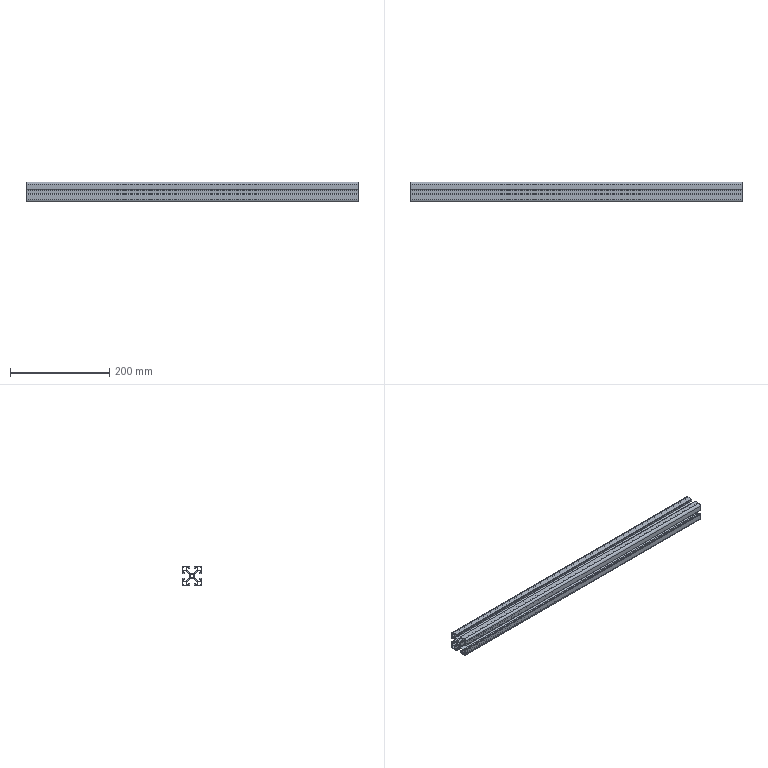Part | STEP file | MK-8-4040C-L-00 profile 4040C standard 670mm | 1 solid | 188 faces | box 670 x 40 x 40 mm | volume 320427 mm3 | cylinder 94 | plane 94 | commonest cylinder face diameters 0.6 x30 2 x28 4 x16 0.4 x8 6 x4 9 x4